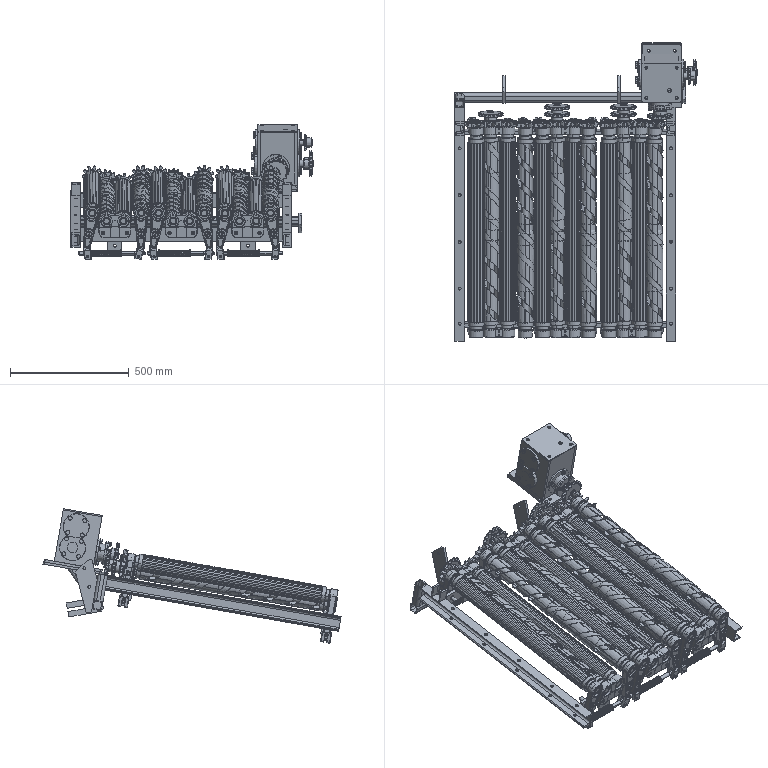Part | SolidWorks | features LayoutProfileFeature 1 | 319 solids | 13404 faces | volume 51530295 mm3 | cylinder 5742 | plane 3254 | spline 2592 | cone 1816 | commonest cylinder face diameters 4 x654 70 x348 76.673 x264 65 x254 19.857 x238 31.085 x224